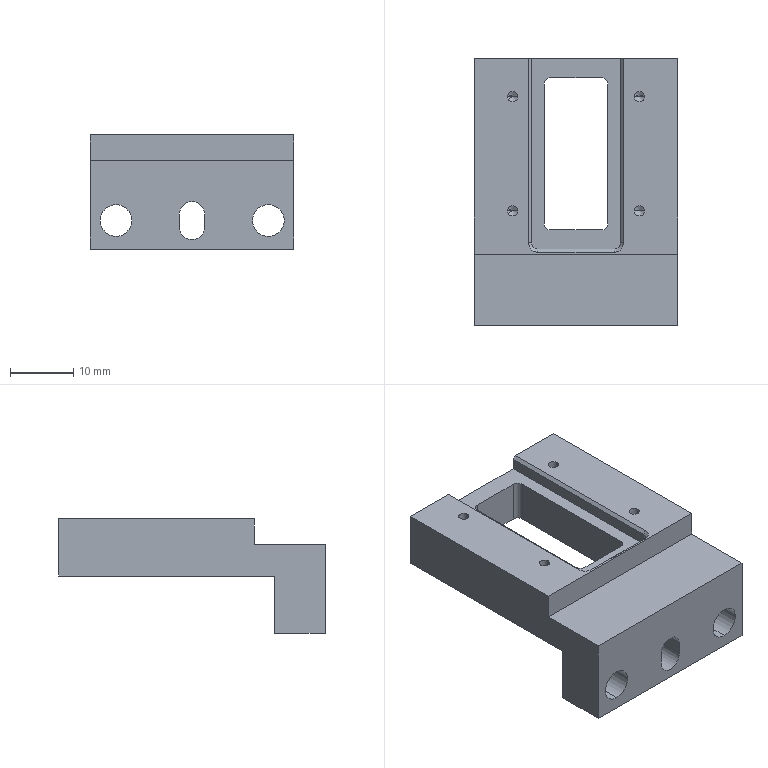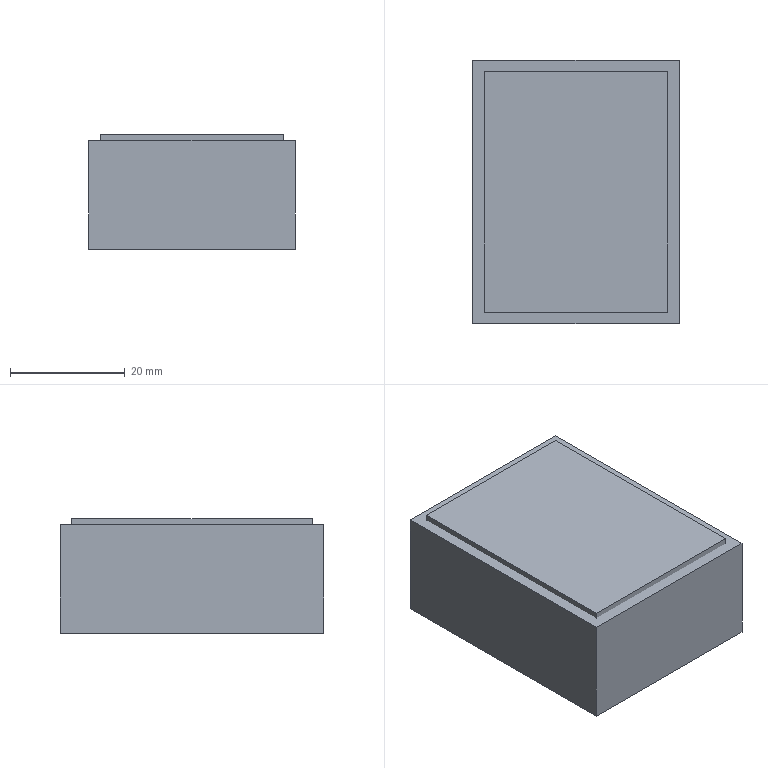CAM job | NX | 3+2 milling, drilling | part box 32 x 42 x 18 mm | stock box 36 x 46 x 20 mm
Tools:
number,name,description,diameter,corner_radius,flute_length,length,flutes
11,D10JING,Milling Tool-5 Parameters,10.0,0.0,50.0,75.0,2
7,D6A45,Milling Tool-5 Parameters,6.0,0.0,50.0,75.0,2
14,1.6ZT,Drilling Tool,1.6,0.0,35.0,50.0,2
10,D10,Milling Tool-5 Parameters,10.0,0.0,50.0,75.0,2
6,D6,Milling Tool-5 Parameters,6.0,0.0,50.0,75.0,2
2,D2,Milling Tool-5 Parameters,2.0,0.0,50.0,75.0,2
13,5.0ZT,Drilling Tool,5.0,0.0,35.0,50.0,2
3,D3,Milling Tool-5 Parameters,3.0,0.0,50.0,75.0,2
Operations:
program,operation,operation_type,tool,method,geometry_group,spindle_rpm,surface_speed,feed_per_tooth,feed_cut,feed_plunge,cut_length_mm,path_length_mm,cut_time_min,machine_time_min
1,FLOOR_WALL,VolumeBased25DMillingOperation,D10JING,METHOD,A,9500.0,298.0,0.0658,1250.0,100.0,491.997,545.997,0.3936,0.399
1,DRILLING,Operation,D6A45,METHOD,A,5000.0,94.0,0.025,250.0,0.0,16.0,157.72,0.064,0.0782
1,DRILLING_COPY,Operation,1.6ZT,METHOD,A,2009.0,10.0,0.0249,100.0,0.0,34.723,195.166,0.3472,0.3633
1,ZLEVEL_PROFILE,ZLevelMilling,D10,METHOD,A,9500.0,298.0,0.1579,3000.0,1000.0,6549.892,6624.792,2.209,2.216
1,ZLEVEL_PROFILE_COPY_1,ZLevelMilling,D10JING,METHOD,A,9500.0,298.0,0.0632,1200.0,1000.0,187.754,280.554,0.1571,0.1664
1,FLOOR_WALL_1,VolumeBased25DMillingOperation,D6,METHOD,A,9500.0,179.0,0.1316,2500.0,1000.0,1195.912,1312.103,0.5094,0.521
1,FLOOR_WALL_1_COPY,VolumeBased25DMillingOperation,D6,METHOD,A,9500.0,179.0,0.1316,2500.0,1000.0,633.664,720.565,0.2694,0.2781
1,ZLEVEL_PROFILE_COPY,ZLevelMilling,D6,METHOD,A,9500.0,179.0,0.1158,2200.0,1000.0,670.682,738.982,0.3255,0.3323
1,FLOOR_WALL_1_1,VolumeBased25DMillingOperation,D6,METHOD,A,9500.0,298.0,0.0658,1250.0,100.0,254.246,377.447,0.2034,0.2157
1,FLOOR_WALL_1_1_COPY,VolumeBased25DMillingOperation,D6,METHOD,A,9500.0,298.0,0.0658,1250.0,100.0,210.614,289.714,0.1685,0.1764
1,ZLEVEL_PROFILE_COPY_1_COPY,ZLevelMilling,D6,METHOD,A,9500.0,298.0,0.0632,1200.0,1000.0,50.978,125.978,0.0431,0.0506
1,ZLEVEL_PROFILE_COPY_COPY,ZLevelMilling,D2,METHOD,A,9500.0,59.0,0.0526,1000.0,1000.0,176.877,400.898,0.1769,0.1993
1,ZLEVEL_PROFILE_COPY_COPY_COPY,ZLevelMilling,D2,METHOD,A,9500.0,59.0,0.0526,1000.0,1000.0,998.028,1859.424,0.998,1.084
1,PLANAR_MILL_COPY,PlanarMilling,D6A45,METHOD,A,9500.0,179.0,0.0658,1250.0,100.0,195.964,254.964,0.1568,0.1627
1,PLANAR_MILL_COPY_COPY,PlanarMilling,D6A45,METHOD,A,9500.0,179.0,0.0658,1250.0,100.0,56.288,123.288,0.045,0.0517
1,PLANAR_MILL_COPY_COPY_COPY,PlanarMilling,D6A45,METHOD,A,9500.0,179.0,0.0658,1250.0,100.0,40.969,258.91,0.0328,0.0546
1,PLANAR_MILL_COPY_COPY_1,PlanarMilling,D6A45,METHOD,A,9500.0,179.0,0.0658,1250.0,100.0,76.711,136.711,0.0614,0.0674
1,刀补6,VolumeBased25DMillingOperation,D6,METHOD,A,9500.0,298.0,0.0658,1250.0,100.0,75.228,136.828,0.0602,0.0663
2,FLOOR_WALL_COPY,VolumeBased25DMillingOperation,D10JING,METHOD,B,9500.0,298.0,0.0658,1250.0,100.0,807.994,978.398,0.6464,0.6634
2,FLOOR_WALL_1_COPY_1,VolumeBased25DMillingOperation,D6,METHOD,B,9500.0,179.0,0.1316,2500.0,1000.0,5909.203,6308.547,2.433,2.473
2,FLOOR_WALL_1_1_COPY_1,VolumeBased25DMillingOperation,D6,METHOD,B,9500.0,298.0,0.0658,1250.0,100.0,581.046,714.247,0.4648,0.4782
2,PLANAR_MILL_COPY_COPY_2,PlanarMilling,D6A45,METHOD,B,9500.0,179.0,0.0658,1250.0,100.0,91.394,150.394,0.0731,0.079
2,PLANAR_MILL_COPY_COPY_2_COPY,PlanarMilling,D6A45,METHOD,B,9500.0,179.0,0.0658,1250.0,100.0,169.856,344.227,0.1359,0.1533
3,DRILLING_COPY_1,Operation,D6A45,METHOD,C,5000.0,94.0,0.025,250.0,0.0,8.0,103.187,0.032,0.0415
3,DRILLING_COPY_COPY,Operation,5.0ZT,METHOD,C,2000.0,31.0,0.05,200.0,0.0,28.004,143.195,0.14,0.1515
3,ZLEVEL_PROFILE_COPY_COPY_1,ZLevelMilling,D3,METHOD,C,9500.0,89.0,0.0632,1200.0,1000.0,298.777,363.777,0.2544,0.2609
3,PLANAR_MILL_COPY_COPY_3,PlanarMilling,D6A45,METHOD,C,9500.0,179.0,0.0658,1250.0,100.0,53.505,255.165,0.0428,0.063
3,刀补3,ZLevelMilling,D3,METHOD,C,9500.0,89.0,0.0632,1200.0,1000.0,36.67,104.67,0.0308,0.0376